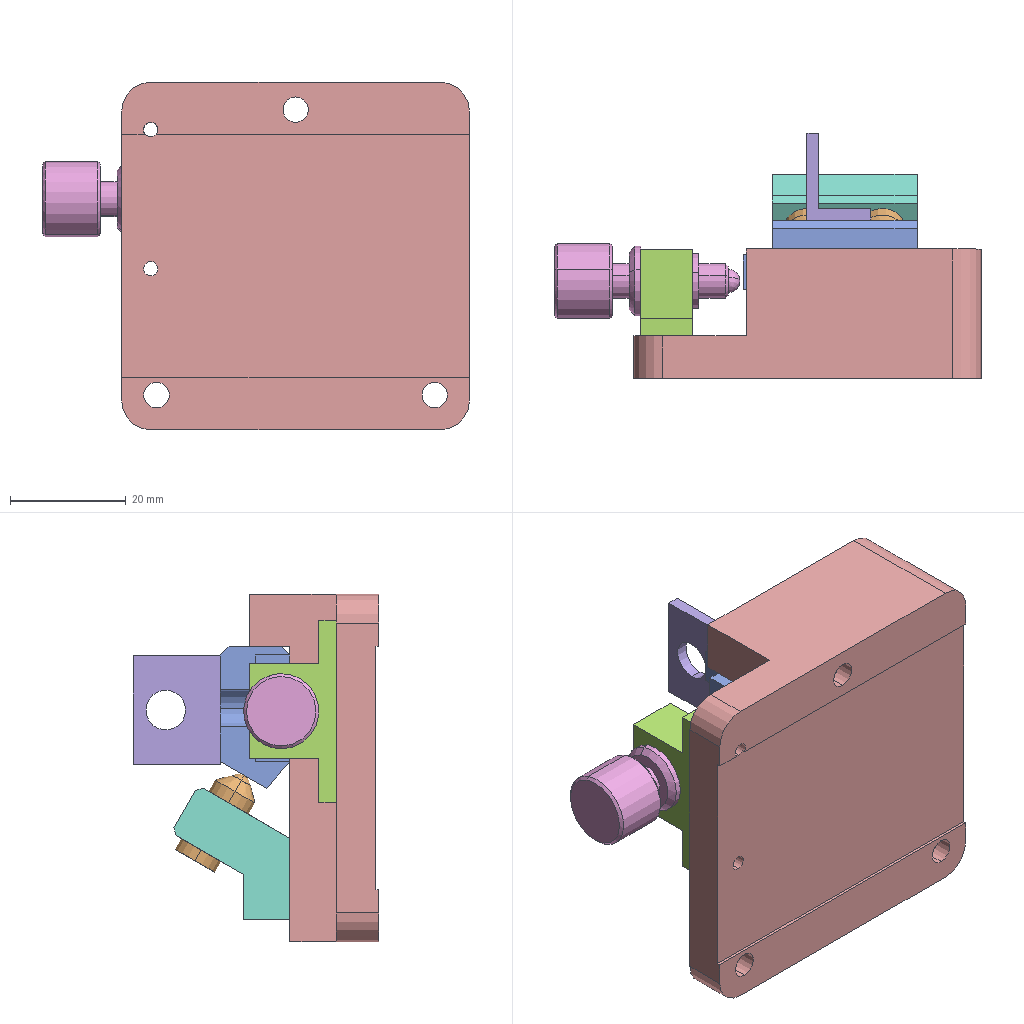Assembly | SolidWorks | 7 different items | 8 placed | box 74 x 42 x 60 mm
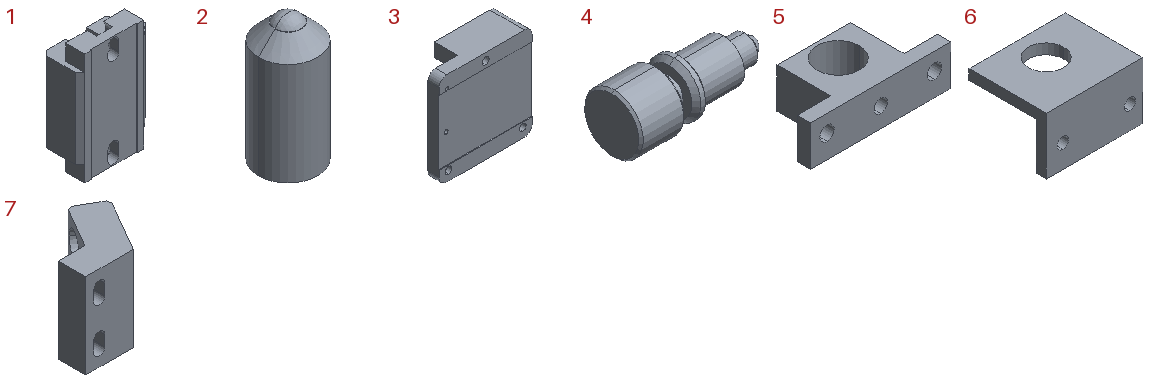Parts list (item | quantity | size | volume | features):
1 | x1 | 24.5 x 12 x 35 mm | 6825 mm3 | features ICE 10, Chamfer 1, Extrusion 1
2 | x2 | 8 x 8 x 17 mm | 759.813 mm3 | features Chamfer 1, Extrusion 1, Revolution 1
3 | x1 | 60 x 22.3 x 60 mm | 44842 mm3 | features ICE 5, HoleWzd 2, Extrusion 1, Fillet 1
4 | x1 | 32 x 13 x 13 mm | 2468 mm3 | features Revolution 1
5 | x1 | 31.4 x 15 x 9 mm | 1899 mm3 | features ICE 7, Extrusion 1
6 | x1 | 18.701 x 15 x 11.037 mm | 809.541 mm3 | features Extrusion 1, ICE 1
7 | x1 | 22.618 x 20.004 x 25 mm | 4524 mm3 | features ICE 15, MoveFace 2, Chamfer 1, Extrusion 1
Mates (type | each side: item.copy, entity, surface, feature):
Coincident | 3.1 face plane Boss-Extrude1 | 1.1 face plane Boss-Extrude1
Concentric | 3.1 face cylinder M3 Tapped Hole1 | 5.1 edge
Coincident | 3.1 face plane Boss-Extrude2 | 5.1 face plane Boss-Extrude1
Concentric | 3.1 face cylinder M3 Tapped Hole1 | 5.1 face cylinder Cut-Extrude2
Slot | 3.1 face cylinder M3 Tapped Hole2 | 1.1 face plane Cut-Extrude12 | 2 times
Concentric | 5.1 face cylinder Cut-Extrude1 | 4.1 face cylinder Revolve1
Coincident | 5.1 face plane Cut-Extrude4 | 4.1 face plane Revolve1
Coincident | 3.1 face plane Boss-Extrude1 | 7.1 face plane Cut-Extrude13
Slot | 3.1 face cylinder M3 Tapped Hole2 | 7.1 face plane Cut-Extrude17 | 2 times
Concentric | 7.1 face cylinder Cut-Extrude2 | 2.1 face cylinder Boss-Extrude1
Tangent | 1.1 face plane Cut-Extrude1 | 2.1 face sphere Revolve2
Concentric | 7.1 face cylinder Cut-Extrude2 | 2.2 face cylinder Boss-Extrude1
Tangent | 1.1 face plane Cut-Extrude1 | 2.2 face sphere Revolve2
Coincident | 1.1 face plane Boss-Extrude1 | 6.1 face plane Boss-Extrude1
Concentric | 1.1 face cylinder Cut-Extrude11 | 6.1 face cylinder Boss-Extrude1 | 2 times